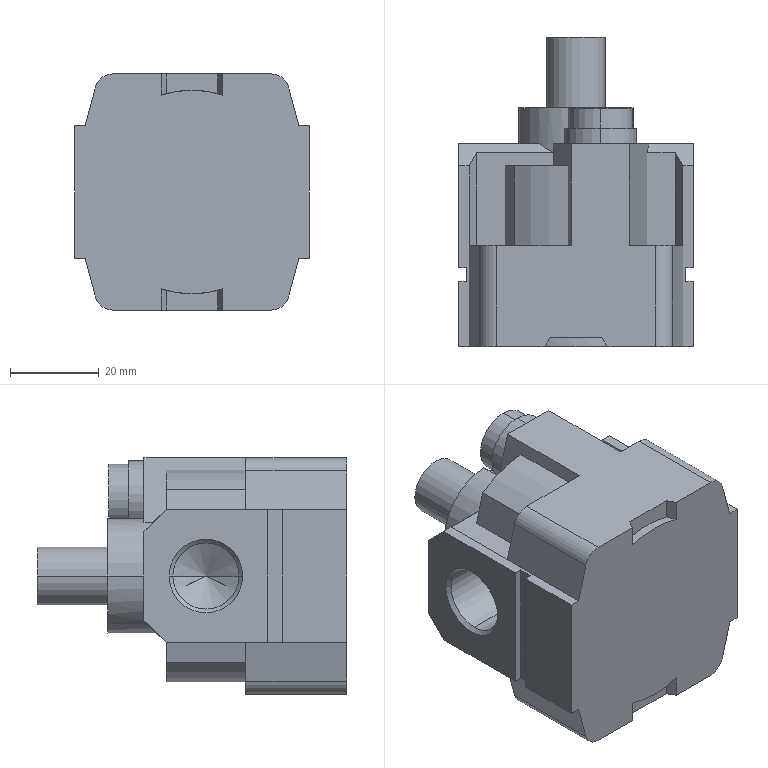Part | STEP file | 11-GY_AL30-03-A(0)_BODY-30-V10-22111.11 | 1 solid | 119 faces | box 53 x 69.9 x 53.4 mm | volume 106073 mm3 | plane 65 | cylinder 30 | cone 24 | commonest cylinder face diameters 3.242 x8 8 x4 14.95 x4 26 x3 13.2 x2 14.5 x2